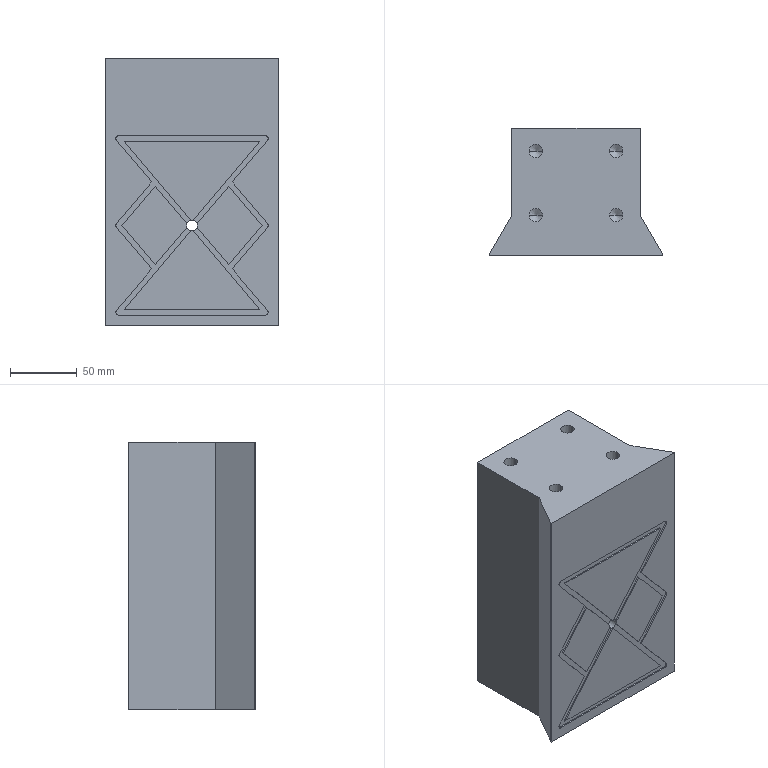Part | STEP file | DAU BUA_3 | 1 solid | 83 faces | box 130 x 95 x 200 mm | volume 1901919 mm3 | plane 39 | cylinder 26 | cone 18 | commonest cylinder face diameters 8.376 x8 10.106 x8 4 x6 8 x2 15 x2